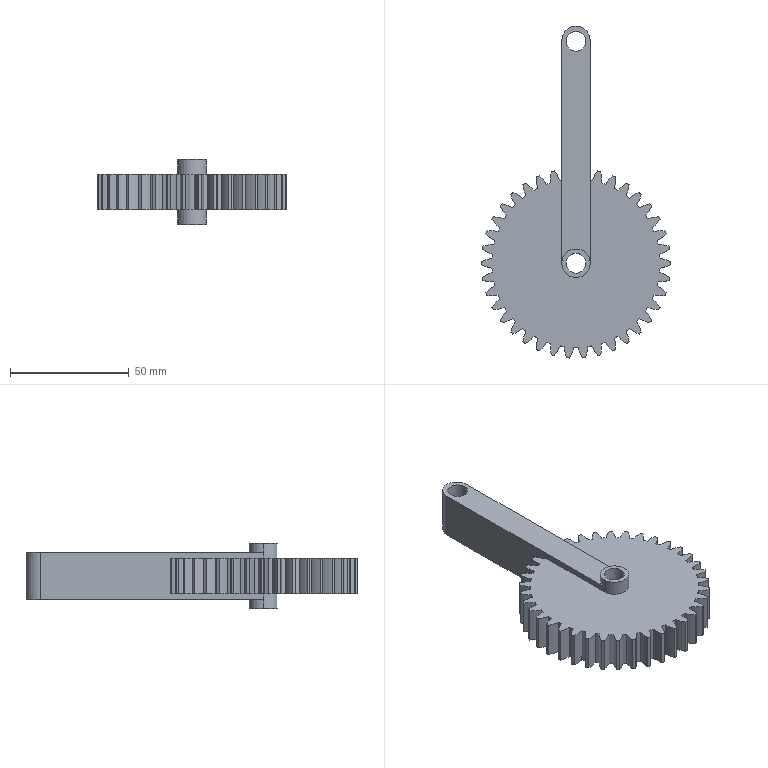Part | SolidWorks | features ICE 3, Extrusion 1, Fillet 1 | 1 solid | 168 faces | box 80 x 139.91 x 27.4 mm | volume 82359 mm3 | cylinder 160 | plane 8 | commonest cylinder face diameters 30.4 x76 70.998 x37 80 x37 12 x6 8.382 x4